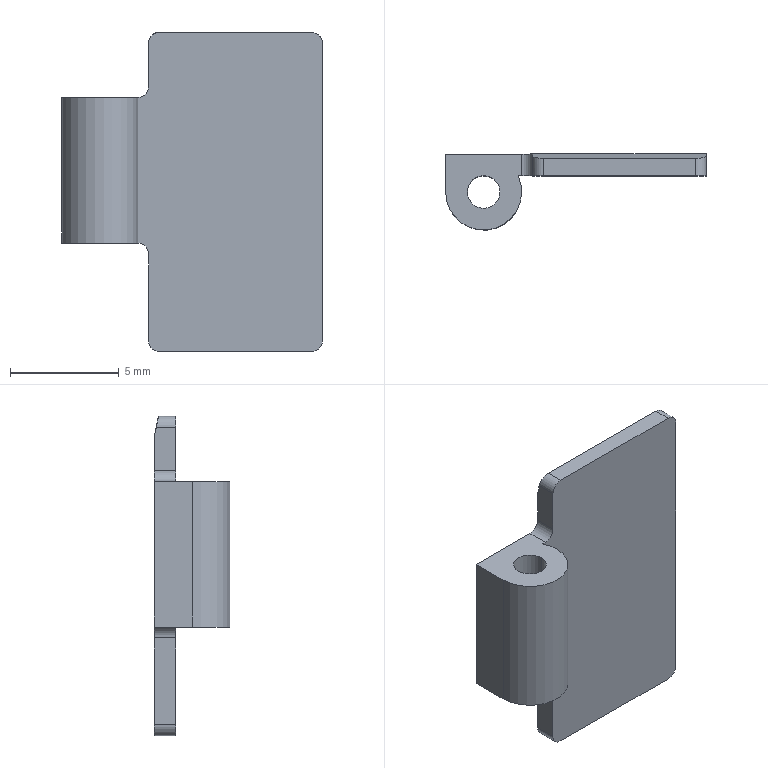Part | SolidWorks | features ICE 5, Chamfer 1, Extrusion 1, Fillet 1 | 1 solid | 20 faces | box 12 x 3.5 x 14.7 mm | volume 181.213 mm3 | plane 11 | cylinder 9 | commonest cylinder face diameters 1 x6 1.5 x2 3.5 x1
STEP:
#1=CARTESIAN_POINT('',(-0.75,0.,0.));
#2=VERTEX_POINT('',#1);
#3=CARTESIAN_POINT('',(0.75,0.,0.));
#4=VERTEX_POINT('',#3);
#5=CARTESIAN_POINT('',(0.,0.,0.));
#6=DIRECTION('',(0.,0.,1.));
#7=DIRECTION('',(1.,0.,0.));
#8=AXIS2_PLACEMENT_3D('',#5,#6,#7);
#9=CIRCLE('',#8,0.75);
#10=EDGE_CURVE('',#2,#4,#9,.T.);
#11=ORIENTED_EDGE('',*,*,#10,.F.);
#12=CARTESIAN_POINT('',(-0.75,0.,6.7));
#13=VERTEX_POINT('',#12);
#14=CARTESIAN_POINT('',(-0.75,0.,0.));
#15=DIRECTION('',(0.,0.,1.));
#16=VECTOR('',#15,1000.);
#17=LINE('',#14,#16);
#18=EDGE_CURVE('',#2,#13,#17,.T.);
#19=ORIENTED_EDGE('',*,*,#18,.T.);
#20=CARTESIAN_POINT('',(0.75,0.,6.7));
#21=VERTEX_POINT('',#20);
#22=CARTESIAN_POINT('',(0.,0.,6.7));
#23=DIRECTION('',(0.,0.,1.));
#24=DIRECTION('',(1.,0.,0.));
#25=AXIS2_PLACEMENT_3D('',#22,#23,#24);
#26=CIRCLE('',#25,0.75);
#27=EDGE_CURVE('',#13,#21,#26,.T.);
#28=ORIENTED_EDGE('',*,*,#27,.T.);
#29=CARTESIAN_POINT('',(0.75,0.,0.));
#30=DIRECTION('',(0.,0.,1.));
#31=VECTOR('',#30,1000.);
#32=LINE('',#29,#31);
#33=EDGE_CURVE('',#4,#21,#32,.T.);
#34=ORIENTED_EDGE('',*,*,#33,.F.);
#35=EDGE_LOOP('',(#11,#19,#28,#34));
#36=FACE_OUTER_BOUND('',#35,.T.);
#37=CARTESIAN_POINT('',(0.,0.,0.));
#38=DIRECTION('',(0.,0.,1.));
#39=DIRECTION('',(1.,0.,0.));
#40=AXIS2_PLACEMENT_3D('',#37,#38,#39);
#41=CYLINDRICAL_SURFACE('',#40,0.75);
#42=ADVANCED_FACE('',(#36),#41,.F.);
#43=CARTESIAN_POINT('',(0.,0.,0.));
#44=DIRECTION('',(0.,0.,1.));
#45=DIRECTION('',(1.,0.,0.));
#46=AXIS2_PLACEMENT_3D('',#43,#44,#45);
#47=CIRCLE('',#46,0.75);
#48=EDGE_CURVE('',#4,#2,#47,.T.);
#49=ORIENTED_EDGE('',*,*,#48,.T.);
#50=ORIENTED_EDGE('',*,*,#10,.T.);
#51=EDGE_LOOP('',(#49,#50));
#52=FACE_BOUND('',#51,.T.);
#53=CARTESIAN_POINT('',(1.75,1.75,0.));
#54=VERTEX_POINT('',#53);
#55=CARTESIAN_POINT('',(-1.75,1.75,0.));
#56=VERTEX_POINT('',#55);
#57=CARTESIAN_POINT('',(-1.75,1.75,0.));
#58=DIRECTION('',(-1.,0.,0.));
#59=VECTOR('',#58,1000.);
#60=LINE('',#57,#59);
#61=EDGE_CURVE('',#54,#56,#60,.T.);
#62=ORIENTED_EDGE('',*,*,#61,.F.);
#63=CARTESIAN_POINT('',(1.75,0.75,0.));
#64=VERTEX_POINT('',#63);
#65=CARTESIAN_POINT('',(1.75,0.75,0.));
#66=DIRECTION('',(0.,-1.,0.));
#67=VECTOR('',#66,1000.);
#68=LINE('',#65,#67);
#69=EDGE_CURVE('',#54,#64,#68,.T.);
#70=ORIENTED_EDGE('',*,*,#69,.T.);
#71=CARTESIAN_POINT('',(1.581,0.75,0.));
#72=VERTEX_POINT('',#71);
#73=CARTESIAN_POINT('',(-1.75,0.75,0.));
#74=DIRECTION('',(-1.,0.,0.));
#75=VECTOR('',#74,1000.);
#76=LINE('',#73,#75);
#77=EDGE_CURVE('',#64,#72,#76,.T.);
#78=ORIENTED_EDGE('',*,*,#77,.T.);
#79=CARTESIAN_POINT('',(-1.75,0.,0.));
#80=VERTEX_POINT('',#79);
#81=CARTESIAN_POINT('',(0.,0.,0.));
#82=DIRECTION('',(0.,0.,1.));
#83=DIRECTION('',(1.,0.,0.));
#84=AXIS2_PLACEMENT_3D('',#81,#82,#83);
#85=CIRCLE('',#84,1.75);
#86=EDGE_CURVE('',#80,#72,#85,.T.);
#87=ORIENTED_EDGE('',*,*,#86,.F.);
#88=CARTESIAN_POINT('',(-1.75,0.75,0.));
#89=DIRECTION('',(0.,1.,0.));
#90=VECTOR('',#89,1000.);
#91=LINE('',#88,#90);
#92=EDGE_CURVE('',#80,#56,#91,.T.);
#93=ORIENTED_EDGE('',*,*,#92,.T.);
#94=EDGE_LOOP('',(#62,#70,#78,#87,#93));
#95=FACE_OUTER_BOUND('',#94,.T.);
#96=CARTESIAN_POINT('',(0.,0.,0.));
#97=DIRECTION('',(0.,0.,1.));
#98=DIRECTION('',(1.,0.,0.));
#99=AXIS2_PLACEMENT_3D('',#96,#97,#98);
#100=PLANE('',#99);
#101=ADVANCED_FACE('',(#52,#95),#100,.F.);
#102=CARTESIAN_POINT('',(-1.75,0.,6.7));
#103=VERTEX_POINT('',#102);
#104=CARTESIAN_POINT('',(1.581,0.75,6.7));
#105=VERTEX_POINT('',#104);
#106=CARTESIAN_POINT('',(0.,0.,6.7));
#107=DIRECTION('',(0.,0.,1.));
#108=DIRECTION('',(1.,0.,0.));
#109=AXIS2_PLACEMENT_3D('',#106,#107,#108);
#110=CIRCLE('',#109,1.75);
#111=EDGE_CURVE('',#103,#105,#110,.T.);
#112=ORIENTED_EDGE('',*,*,#111,.F.);
#113=CARTESIAN_POINT('',(-1.75,0.,-0.7688));
#114=DIRECTION('',(0.,0.,1.));
#115=VECTOR('',#114,1000.);
#116=LINE('',#113,#115);
#117=EDGE_CURVE('',#80,#103,#116,.T.);
#118=ORIENTED_EDGE('',*,*,#117,.F.);
#119=ORIENTED_EDGE('',*,*,#86,.T.);
#120=CARTESIAN_POINT('',(1.581,0.75,6.7));
#121=DIRECTION('',(0.,0.,-1.));
#122=VECTOR('',#121,1000.);
#123=LINE('',#120,#122);
#124=EDGE_CURVE('',#105,#72,#123,.T.);
#125=ORIENTED_EDGE('',*,*,#124,.F.);
#126=EDGE_LOOP('',(#112,#118,#119,#125));
#127=FACE_OUTER_BOUND('',#126,.T.);
#128=CARTESIAN_POINT('',(0.,0.,6.7));
#129=DIRECTION('',(0.,0.,-1.));
#130=DIRECTION('',(-1.,0.,0.));
#131=AXIS2_PLACEMENT_3D('',#128,#129,#130);
#132=CYLINDRICAL_SURFACE('',#131,1.75);
#133=ADVANCED_FACE('',(#127),#132,.T.);
#134=CARTESIAN_POINT('',(1.75,0.75,6.7));
#135=VERTEX_POINT('',#134);
#136=CARTESIAN_POINT('',(-1.75,0.75,6.7));
#137=DIRECTION('',(1.,0.,0.));
#138=VECTOR('',#137,1000.);
#139=LINE('',#136,#138);
#140=EDGE_CURVE('',#105,#135,#139,.T.);
#141=ORIENTED_EDGE('',*,*,#140,.T.);
#142=CARTESIAN_POINT('',(1.75,1.75,6.7));
#143=VERTEX_POINT('',#142);
#144=CARTESIAN_POINT('',(1.75,0.,6.7));
#145=DIRECTION('',(0.,1.,0.));
#146=VECTOR('',#145,1000.);
#147=LINE('',#144,#146);
#148=EDGE_CURVE('',#135,#143,#147,.T.);
#149=ORIENTED_EDGE('',*,*,#148,.T.);
#150=CARTESIAN_POINT('',(-1.75,1.75,6.7));
#151=VERTEX_POINT('',#150);
#152=CARTESIAN_POINT('',(-1.75,1.75,6.7));
#153=DIRECTION('',(1.,0.,0.));
#154=VECTOR('',#153,1000.);
#155=LINE('',#152,#154);
#156=EDGE_CURVE('',#151,#143,#155,.T.);
#157=ORIENTED_EDGE('',*,*,#156,.F.);
#158=CARTESIAN_POINT('',(-1.75,0.75,6.7));
#159=DIRECTION('',(0.,1.,0.));
#160=VECTOR('',#159,1000.);
#161=LINE('',#158,#160);
#162=EDGE_CURVE('',#103,#151,#161,.T.);
#163=ORIENTED_EDGE('',*,*,#162,.F.);
#164=ORIENTED_EDGE('',*,*,#111,.T.);
#165=EDGE_LOOP('',(#141,#149,#157,#163,#164));
#166=FACE_OUTER_BOUND('',#165,.T.);
#167=CARTESIAN_POINT('',(0.,0.,6.7));
#168=DIRECTION('',(0.,0.,1.));
#169=DIRECTION('',(1.,0.,0.));
#170=AXIS2_PLACEMENT_3D('',#167,#168,#169);
#171=CIRCLE('',#170,0.75);
#172=EDGE_CURVE('',#21,#13,#171,.T.);
#173=ORIENTED_EDGE('',*,*,#172,.F.);
#174=ORIENTED_EDGE('',*,*,#27,.F.);
#175=EDGE_LOOP('',(#173,#174));
#176=FACE_BOUND('',#175,.T.);
#177=CARTESIAN_POINT('',(0.,0.,6.7));
#178=DIRECTION('',(0.,0.,1.));
#179=DIRECTION('',(1.,0.,0.));
#180=AXIS2_PLACEMENT_3D('',#177,#178,#179);
#181=PLANE('',#180);
#182=ADVANCED_FACE('',(#166,#176),#181,.T.);
#183=ORIENTED_EDGE('',*,*,#18,.F.);
#184=ORIENTED_EDGE('',*,*,#48,.F.);
#185=ORIENTED_EDGE('',*,*,#33,.T.);
#186=ORIENTED_EDGE('',*,*,#172,.T.);
#187=EDGE_LOOP('',(#183,#184,#185,#186));
#188=FACE_OUTER_BOUND('',#187,.T.);
#189=CARTESIAN_POINT('',(0.,0.,0.));
#190=DIRECTION('',(0.,0.,1.));
#191=DIRECTION('',(1.,0.,0.));
#192=AXIS2_PLACEMENT_3D('',#189,#190,#191);
#193=CYLINDRICAL_SURFACE('',#192,0.75);
#194=ADVANCED_FACE('',(#188),#193,.F.);
#195=CARTESIAN_POINT('',(2.75,1.75,-5.));
#196=VERTEX_POINT('',#195);
#197=CARTESIAN_POINT('',(9.75,1.75,-5.));
#198=VERTEX_POINT('',#197);
#199=CARTESIAN_POINT('',(2.25,1.75,-5.));
#200=DIRECTION('',(1.,0.,0.));
#201=VECTOR('',#200,1000.);
#202=LINE('',#199,#201);
#203=EDGE_CURVE('',#196,#198,#202,.T.);
#204=ORIENTED_EDGE('',*,*,#203,.F.);
#205=CARTESIAN_POINT('',(2.25,1.75,-4.5));
#206=VERTEX_POINT('',#205);
#207=CARTESIAN_POINT('',(2.75,1.75,-4.5));
#208=DIRECTION('',(0.,1.,0.));
#209=DIRECTION('',(0.,0.,1.));
#210=AXIS2_PLACEMENT_3D('',#207,#208,#209);
#211=CIRCLE('',#210,0.5);
#212=EDGE_CURVE('',#196,#206,#211,.T.);
#213=ORIENTED_EDGE('',*,*,#212,.T.);
#214=CARTESIAN_POINT('',(2.25,1.75,-0.5));
#215=VERTEX_POINT('',#214);
#216=CARTESIAN_POINT('',(2.25,1.75,-5.));
#217=DIRECTION('',(0.,0.,1.));
#218=VECTOR('',#217,1000.);
#219=LINE('',#216,#218);
#220=EDGE_CURVE('',#206,#215,#219,.T.);
#221=ORIENTED_EDGE('',*,*,#220,.T.);
#222=CARTESIAN_POINT('',(1.75,1.75,-0.5));
#223=DIRECTION('',(0.,-1.,0.));
#224=DIRECTION('',(0.,0.,1.));
#225=AXIS2_PLACEMENT_3D('',#222,#223,#224);
#226=CIRCLE('',#225,0.5);
#227=EDGE_CURVE('',#215,#54,#226,.T.);
#228=ORIENTED_EDGE('',*,*,#227,.T.);
#229=ORIENTED_EDGE('',*,*,#61,.T.);
#230=CARTESIAN_POINT('',(-1.75,1.75,0.));
#231=DIRECTION('',(0.,0.,1.));
#232=VECTOR('',#231,1000.);
#233=LINE('',#230,#232);
#234=EDGE_CURVE('',#56,#151,#233,.T.);
#235=ORIENTED_EDGE('',*,*,#234,.T.);
#236=ORIENTED_EDGE('',*,*,#156,.T.);
#237=CARTESIAN_POINT('',(2.25,1.75,7.2));
#238=VERTEX_POINT('',#237);
#239=CARTESIAN_POINT('',(1.75,1.75,7.2));
#240=DIRECTION('',(0.,-1.,0.));
#241=DIRECTION('',(0.,0.,1.));
#242=AXIS2_PLACEMENT_3D('',#239,#240,#241);
#243=CIRCLE('',#242,0.5);
#244=EDGE_CURVE('',#143,#238,#243,.T.);
#245=ORIENTED_EDGE('',*,*,#244,.T.);
#246=CARTESIAN_POINT('',(2.25,1.75,8.7));
#247=VERTEX_POINT('',#246);
#248=CARTESIAN_POINT('',(2.25,1.75,9.7));
#249=DIRECTION('',(0.,0.,-1.));
#250=VECTOR('',#249,1000.);
#251=LINE('',#248,#250);
#252=EDGE_CURVE('',#247,#238,#251,.T.);
#253=ORIENTED_EDGE('',*,*,#252,.F.);
#254=CARTESIAN_POINT('',(10.25,1.75,8.7));
#255=VERTEX_POINT('',#254);
#256=CARTESIAN_POINT('',(10.25,1.75,8.7));
#257=DIRECTION('',(1.,0.,0.));
#258=VECTOR('',#257,1000.);
#259=LINE('',#256,#258);
#260=EDGE_CURVE('',#247,#255,#259,.T.);
#261=ORIENTED_EDGE('',*,*,#260,.T.);
#262=CARTESIAN_POINT('',(10.25,1.75,-4.5));
#263=VERTEX_POINT('',#262);
#264=CARTESIAN_POINT('',(10.25,1.75,0.));
#265=DIRECTION('',(0.,0.,-1.));
#266=VECTOR('',#265,1000.);
#267=LINE('',#264,#266);
#268=EDGE_CURVE('',#255,#263,#267,.T.);
#269=ORIENTED_EDGE('',*,*,#268,.T.);
#270=CARTESIAN_POINT('',(9.75,1.75,-4.5));
#271=DIRECTION('',(0.,1.,0.));
#272=DIRECTION('',(0.,0.,1.));
#273=AXIS2_PLACEMENT_3D('',#270,#271,#272);
#274=CIRCLE('',#273,0.5);
#275=EDGE_CURVE('',#263,#198,#274,.T.);
#276=ORIENTED_EDGE('',*,*,#275,.T.);
#277=EDGE_LOOP('',(#204,#213,#221,#228,#229,#235,#236,#245,#253,#261,#269,#276));
#278=FACE_OUTER_BOUND('',#277,.T.);
#279=CARTESIAN_POINT('',(0.,1.75,0.));
#280=DIRECTION('',(0.,1.,0.));
#281=DIRECTION('',(0.,0.,1.));
#282=AXIS2_PLACEMENT_3D('',#279,#280,#281);
#283=PLANE('',#282);
#284=ADVANCED_FACE('',(#278),#283,.T.);
#285=CARTESIAN_POINT('',(10.25,0.75,9.2));
#286=VERTEX_POINT('',#285);
#287=CARTESIAN_POINT('',(10.25,0.75,-4.5));
#288=VERTEX_POINT('',#287);
#289=CARTESIAN_POINT('',(10.25,0.75,0.));
#290=DIRECTION('',(0.,0.,-1.));
#291=VECTOR('',#290,1000.);
#292=LINE('',#289,#291);
#293=EDGE_CURVE('',#286,#288,#292,.T.);
#294=ORIENTED_EDGE('',*,*,#293,.F.);
#295=CARTESIAN_POINT('',(9.75,0.75,9.7));
#296=VERTEX_POINT('',#295);
#297=CARTESIAN_POINT('',(9.75,0.75,9.2));
#298=DIRECTION('',(0.,-1.,0.));
#299=DIRECTION('',(0.,0.,1.));
#300=AXIS2_PLACEMENT_3D('',#297,#298,#299);
#301=CIRCLE('',#300,0.5);
#302=EDGE_CURVE('',#286,#296,#301,.T.);
#303=ORIENTED_EDGE('',*,*,#302,.T.);
#304=CARTESIAN_POINT('',(2.75,0.75,9.7));
#305=VERTEX_POINT('',#304);
#306=CARTESIAN_POINT('',(10.25,0.75,9.7));
#307=DIRECTION('',(1.,0.,0.));
#308=VECTOR('',#307,1000.);
#309=LINE('',#306,#308);
#310=EDGE_CURVE('',#305,#296,#309,.T.);
#311=ORIENTED_EDGE('',*,*,#310,.F.);
#312=CARTESIAN_POINT('',(2.25,0.75,9.2));
#313=VERTEX_POINT('',#312);
#314=CARTESIAN_POINT('',(2.75,0.75,9.2));
#315=DIRECTION('',(0.,-1.,0.));
#316=DIRECTION('',(0.,0.,1.));
#317=AXIS2_PLACEMENT_3D('',#314,#315,#316);
#318=CIRCLE('',#317,0.5);
#319=EDGE_CURVE('',#305,#313,#318,.T.);
#320=ORIENTED_EDGE('',*,*,#319,.T.);
#321=CARTESIAN_POINT('',(2.25,0.75,7.2));
#322=VERTEX_POINT('',#321);
#323=CARTESIAN_POINT('',(2.25,0.75,9.7));
#324=DIRECTION('',(0.,0.,-1.));
#325=VECTOR('',#324,1000.);
#326=LINE('',#323,#325);
#327=EDGE_CURVE('',#313,#322,#326,.T.);
#328=ORIENTED_EDGE('',*,*,#327,.T.);
#329=CARTESIAN_POINT('',(1.75,0.75,7.2));
#330=DIRECTION('',(0.,1.,0.));
#331=DIRECTION('',(0.,0.,1.));
#332=AXIS2_PLACEMENT_3D('',#329,#330,#331);
#333=CIRCLE('',#332,0.5);
#334=EDGE_CURVE('',#322,#135,#333,.T.);
#335=ORIENTED_EDGE('',*,*,#334,.T.);
#336=ORIENTED_EDGE('',*,*,#140,.F.);
#337=ORIENTED_EDGE('',*,*,#124,.T.);
#338=ORIENTED_EDGE('',*,*,#77,.F.);
#339=CARTESIAN_POINT('',(2.25,0.75,-0.5));
#340=VERTEX_POINT('',#339);
#341=CARTESIAN_POINT('',(1.75,0.75,-0.5));
#342=DIRECTION('',(0.,1.,0.));
#343=DIRECTION('',(0.,0.,1.));
#344=AXIS2_PLACEMENT_3D('',#341,#342,#343);
#345=CIRCLE('',#344,0.5);
#346=EDGE_CURVE('',#64,#340,#345,.T.);
#347=ORIENTED_EDGE('',*,*,#346,.T.);
#348=CARTESIAN_POINT('',(2.25,0.75,-4.5));
#349=VERTEX_POINT('',#348);
#350=CARTESIAN_POINT('',(2.25,0.75,-5.));
#351=DIRECTION('',(0.,0.,1.));
#352=VECTOR('',#351,1000.);
#353=LINE('',#350,#352);
#354=EDGE_CURVE('',#349,#340,#353,.T.);
#355=ORIENTED_EDGE('',*,*,#354,.F.);
#356=CARTESIAN_POINT('',(2.75,0.75,-5.));
#357=VERTEX_POINT('',#356);
#358=CARTESIAN_POINT('',(2.75,0.75,-4.5));
#359=DIRECTION('',(0.,-1.,0.));
#360=DIRECTION('',(0.,0.,1.));
#361=AXIS2_PLACEMENT_3D('',#358,#359,#360);
#362=CIRCLE('',#361,0.5);
#363=EDGE_CURVE('',#349,#357,#362,.T.);
#364=ORIENTED_EDGE('',*,*,#363,.T.);
#365=CARTESIAN_POINT('',(9.75,0.75,-5.));
#366=VERTEX_POINT('',#365);
#367=CARTESIAN_POINT('',(10.25,0.75,-5.));
#368=DIRECTION('',(-1.,0.,0.));
#369=VECTOR('',#368,1000.);
#370=LINE('',#367,#369);
#371=EDGE_CURVE('',#366,#357,#370,.T.);
#372=ORIENTED_EDGE('',*,*,#371,.F.);
#373=CARTESIAN_POINT('',(9.75,0.75,-4.5));
#374=DIRECTION('',(0.,-1.,0.));
#375=DIRECTION('',(0.,0.,1.));
#376=AXIS2_PLACEMENT_3D('',#373,#374,#375);
#377=CIRCLE('',#376,0.5);
#378=EDGE_CURVE('',#366,#288,#377,.T.);
#379=ORIENTED_EDGE('',*,*,#378,.T.);
#380=EDGE_LOOP('',(#294,#303,#311,#320,#328,#335,#336,#337,#338,#347,#355,#364,#372,#379));
#381=FACE_OUTER_BOUND('',#380,.T.);
#382=CARTESIAN_POINT('',(0.,0.75,0.));
#383=DIRECTION('',(0.,1.,0.));
#384=DIRECTION('',(0.,0.,1.));
#385=AXIS2_PLACEMENT_3D('',#382,#383,#384);
#386=PLANE('',#385);
#387=ADVANCED_FACE('',(#381),#386,.F.);
#388=ORIENTED_EDGE('',*,*,#234,.F.);
#389=ORIENTED_EDGE('',*,*,#92,.F.);
#390=ORIENTED_EDGE('',*,*,#117,.T.);
#391=ORIENTED_EDGE('',*,*,#162,.T.);
#392=EDGE_LOOP('',(#388,#389,#390,#391));
#393=FACE_OUTER_BOUND('',#392,.T.);
#394=CARTESIAN_POINT('',(-1.75,0.75,0.));
#395=DIRECTION('',(-1.,0.,0.));
#396=DIRECTION('',(0.,0.,1.));
#397=AXIS2_PLACEMENT_3D('',#394,#395,#396);
#398=PLANE('',#397);
#399=ADVANCED_FACE('',(#393),#398,.T.);
#400=CARTESIAN_POINT('',(10.25,1.65,9.2));
#401=VERTEX_POINT('',#400);
#402=CARTESIAN_POINT('',(10.25,3.385,0.5269));
#403=DIRECTION('',(0.,-0.1961,0.9806));
#404=VECTOR('',#403,1000.);
#405=LINE('',#402,#404);
#406=EDGE_CURVE('',#255,#401,#405,.T.);
#407=ORIENTED_EDGE('',*,*,#406,.T.);
#408=CARTESIAN_POINT('',(10.25,0.75,9.2));
#409=DIRECTION('',(0.,-1.,0.));
#410=VECTOR('',#409,1000.);
#411=LINE('',#408,#410);
#412=EDGE_CURVE('',#401,#286,#411,.T.);
#413=ORIENTED_EDGE('',*,*,#412,.T.);
#414=ORIENTED_EDGE('',*,*,#293,.T.);
#415=CARTESIAN_POINT('',(10.25,0.75,-4.5));
#416=DIRECTION('',(0.,1.,0.));
#417=VECTOR('',#416,1000.);
#418=LINE('',#415,#417);
#419=EDGE_CURVE('',#288,#263,#418,.T.);
#420=ORIENTED_EDGE('',*,*,#419,.T.);
#421=ORIENTED_EDGE('',*,*,#268,.F.);
#422=EDGE_LOOP('',(#407,#413,#414,#420,#421));
#423=FACE_OUTER_BOUND('',#422,.T.);
#424=CARTESIAN_POINT('',(10.25,0.75,0.));
#425=DIRECTION('',(1.,0.,0.));
#426=DIRECTION('',(0.,0.,-1.));
#427=AXIS2_PLACEMENT_3D('',#424,#425,#426);
#428=PLANE('',#427);
#429=ADVANCED_FACE('',(#423),#428,.T.);
#430=ORIENTED_EDGE('',*,*,#252,.T.);
#431=CARTESIAN_POINT('',(2.25,1.75,7.2));
#432=DIRECTION('',(0.,-1.,0.));
#433=VECTOR('',#432,1000.);
#434=LINE('',#431,#433);
#435=EDGE_CURVE('',#238,#322,#434,.T.);
#436=ORIENTED_EDGE('',*,*,#435,.T.);
#437=ORIENTED_EDGE('',*,*,#327,.F.);
#438=CARTESIAN_POINT('',(2.25,1.65,9.2));
#439=VERTEX_POINT('',#438);
#440=CARTESIAN_POINT('',(2.25,1.75,9.2));
#441=DIRECTION('',(0.,1.,0.));
#442=VECTOR('',#441,1000.);
#443=LINE('',#440,#442);
#444=EDGE_CURVE('',#313,#439,#443,.T.);
#445=ORIENTED_EDGE('',*,*,#444,.T.);
#446=CARTESIAN_POINT('',(2.25,1.55,9.7));
#447=DIRECTION('',(0.,0.1961,-0.9806));
#448=VECTOR('',#447,1000.);
#449=LINE('',#446,#448);
#450=EDGE_CURVE('',#439,#247,#449,.T.);
#451=ORIENTED_EDGE('',*,*,#450,.T.);
#452=EDGE_LOOP('',(#430,#436,#437,#445,#451));
#453=FACE_OUTER_BOUND('',#452,.T.);
#454=CARTESIAN_POINT('',(2.25,1.75,9.7));
#455=DIRECTION('',(1.,0.,0.));
#456=DIRECTION('',(0.,0.,-1.));
#457=AXIS2_PLACEMENT_3D('',#454,#455,#456);
#458=PLANE('',#457);
#459=ADVANCED_FACE('',(#453),#458,.F.);
#460=ORIENTED_EDGE('',*,*,#310,.T.);
#461=CARTESIAN_POINT('',(9.75,1.55,9.7));
#462=VERTEX_POINT('',#461);
#463=CARTESIAN_POINT('',(9.75,1.55,9.7));
#464=DIRECTION('',(0.,1.,0.));
#465=VECTOR('',#464,1000.);
#466=LINE('',#463,#465);
#467=EDGE_CURVE('',#296,#462,#466,.T.);
#468=ORIENTED_EDGE('',*,*,#467,.T.);
#469=CARTESIAN_POINT('',(2.75,1.55,9.7));
#470=VERTEX_POINT('',#469);
#471=CARTESIAN_POINT('',(2.25,1.55,9.7));
#472=DIRECTION('',(-1.,0.,0.));
#473=VECTOR('',#472,1000.);
#474=LINE('',#471,#473);
#475=EDGE_CURVE('',#462,#470,#474,.T.);
#476=ORIENTED_EDGE('',*,*,#475,.T.);
#477=CARTESIAN_POINT('',(2.75,0.,9.7));
#478=DIRECTION('',(0.,-1.,0.));
#479=VECTOR('',#478,1000.);
#480=LINE('',#477,#479);
#481=EDGE_CURVE('',#470,#305,#480,.T.);
#482=ORIENTED_EDGE('',*,*,#481,.T.);
#483=EDGE_LOOP('',(#460,#468,#476,#482));
#484=FACE_OUTER_BOUND('',#483,.T.);
#485=CARTESIAN_POINT('',(0.,0.,9.7));
#486=DIRECTION('',(0.,0.,-1.));
#487=DIRECTION('',(-1.,0.,0.));
#488=AXIS2_PLACEMENT_3D('',#485,#486,#487);
#489=PLANE('',#488);
#490=ADVANCED_FACE('',(#484),#489,.F.);
#491=ORIENTED_EDGE('',*,*,#354,.T.);
#492=CARTESIAN_POINT('',(2.25,1.75,-0.5));
#493=DIRECTION('',(0.,1.,0.));
#494=VECTOR('',#493,1000.);
#495=LINE('',#492,#494);
#496=EDGE_CURVE('',#340,#215,#495,.T.);
#497=ORIENTED_EDGE('',*,*,#496,.T.);
#498=ORIENTED_EDGE('',*,*,#220,.F.);
#499=CARTESIAN_POINT('',(2.25,0.75,-4.5));
#500=DIRECTION('',(0.,-1.,0.));
#501=VECTOR('',#500,1000.);
#502=LINE('',#499,#501);
#503=EDGE_CURVE('',#206,#349,#502,.T.);
#504=ORIENTED_EDGE('',*,*,#503,.T.);
#505=EDGE_LOOP('',(#491,#497,#498,#504));
#506=FACE_OUTER_BOUND('',#505,.T.);
#507=CARTESIAN_POINT('',(2.25,0.75,-5.));
#508=DIRECTION('',(1.,0.,0.));
#509=DIRECTION('',(0.,0.,-1.));
#510=AXIS2_PLACEMENT_3D('',#507,#508,#509);
#511=PLANE('',#510);
#512=ADVANCED_FACE('',(#506),#511,.F.);
#513=ORIENTED_EDGE('',*,*,#371,.T.);
#514=CARTESIAN_POINT('',(2.75,1.75,-5.));
#515=DIRECTION('',(0.,1.,0.));
#516=VECTOR('',#515,1000.);
#517=LINE('',#514,#516);
#518=EDGE_CURVE('',#357,#196,#517,.T.);
#519=ORIENTED_EDGE('',*,*,#518,.T.);
#520=ORIENTED_EDGE('',*,*,#203,.T.);
#521=CARTESIAN_POINT('',(9.75,0.,-5.));
#522=DIRECTION('',(0.,-1.,0.));
#523=VECTOR('',#522,1000.);
#524=LINE('',#521,#523);
#525=EDGE_CURVE('',#198,#366,#524,.T.);
#526=ORIENTED_EDGE('',*,*,#525,.T.);
#527=EDGE_LOOP('',(#513,#519,#520,#526));
#528=FACE_OUTER_BOUND('',#527,.T.);
#529=CARTESIAN_POINT('',(0.,0.,-5.));
#530=DIRECTION('',(0.,0.,-1.));
#531=DIRECTION('',(-1.,0.,0.));
#532=AXIS2_PLACEMENT_3D('',#529,#530,#531);
#533=PLANE('',#532);
#534=ADVANCED_FACE('',(#528),#533,.T.);
#535=ORIENTED_EDGE('',*,*,#475,.F.);
#536=CARTESIAN_POINT('',(9.75,1.55,9.7));
#537=CARTESIAN_POINT('',(10.043,1.55,9.7));
#538=CARTESIAN_POINT('',(10.25,1.591,9.493));
#539=CARTESIAN_POINT('',(10.25,1.65,9.2));
#540=(BOUNDED_CURVE()B_SPLINE_CURVE(3,(#536,#537,#538,#539),.UNSPECIFIED.,.F.,.F.)B_SPLINE_CURVE_WITH_KNOTS((4,4),(0.,1.571),.UNSPECIFIED.)CURVE()GEOMETRIC_REPRESENTATION_ITEM()RATIONAL_B_SPLINE_CURVE((1.,0.8047,0.8047,1.))REPRESENTATION_ITEM(''));
#541=EDGE_CURVE('',#462,#401,#540,.T.);
#542=ORIENTED_EDGE('',*,*,#541,.T.);
#543=ORIENTED_EDGE('',*,*,#406,.F.);
#544=ORIENTED_EDGE('',*,*,#260,.F.);
#545=ORIENTED_EDGE('',*,*,#450,.F.);
#546=CARTESIAN_POINT('',(2.25,1.65,9.2));
#547=CARTESIAN_POINT('',(2.25,1.591,9.493));
#548=CARTESIAN_POINT('',(2.457,1.55,9.7));
#549=CARTESIAN_POINT('',(2.75,1.55,9.7));
#550=(BOUNDED_CURVE()B_SPLINE_CURVE(3,(#546,#547,#548,#549),.UNSPECIFIED.,.F.,.F.)B_SPLINE_CURVE_WITH_KNOTS((4,4),(4.712,6.283),.UNSPECIFIED.)CURVE()GEOMETRIC_REPRESENTATION_ITEM()RATIONAL_B_SPLINE_CURVE((1.,0.8047,0.8047,1.))REPRESENTATION_ITEM(''));
#551=EDGE_CURVE('',#439,#470,#550,.T.);
#552=ORIENTED_EDGE('',*,*,#551,.T.);
#553=EDGE_LOOP('',(#535,#542,#543,#544,#545,#552));
#554=FACE_OUTER_BOUND('',#553,.T.);
#555=CARTESIAN_POINT('',(0.,1.55,9.7));
#556=DIRECTION('',(0.,0.9806,0.1961));
#557=DIRECTION('',(1.,0.,0.));
#558=AXIS2_PLACEMENT_3D('',#555,#556,#557);
#559=PLANE('',#558);
#560=ADVANCED_FACE('',(#554),#559,.T.);
#561=ORIENTED_EDGE('',*,*,#244,.F.);
#562=ORIENTED_EDGE('',*,*,#148,.F.);
#563=ORIENTED_EDGE('',*,*,#334,.F.);
#564=ORIENTED_EDGE('',*,*,#435,.F.);
#565=EDGE_LOOP('',(#561,#562,#563,#564));
#566=FACE_OUTER_BOUND('',#565,.T.);
#567=CARTESIAN_POINT('',(1.75,1.75,7.2));
#568=DIRECTION('',(0.,-1.,0.));
#569=DIRECTION('',(0.,0.,-1.));
#570=AXIS2_PLACEMENT_3D('',#567,#568,#569);
#571=CYLINDRICAL_SURFACE('',#570,0.5);
#572=ADVANCED_FACE('',(#566),#571,.F.);
#573=ORIENTED_EDGE('',*,*,#346,.F.);
#574=ORIENTED_EDGE('',*,*,#69,.F.);
#575=ORIENTED_EDGE('',*,*,#227,.F.);
#576=ORIENTED_EDGE('',*,*,#496,.F.);
#577=EDGE_LOOP('',(#573,#574,#575,#576));
#578=FACE_OUTER_BOUND('',#577,.T.);
#579=CARTESIAN_POINT('',(1.75,0.75,-0.5));
#580=DIRECTION('',(0.,-1.,0.));
#581=DIRECTION('',(0.,0.,-1.));
#582=AXIS2_PLACEMENT_3D('',#579,#580,#581);
#583=CYLINDRICAL_SURFACE('',#582,0.5);
#584=ADVANCED_FACE('',(#578),#583,.F.);
#585=ORIENTED_EDGE('',*,*,#302,.F.);
#586=ORIENTED_EDGE('',*,*,#412,.F.);
#587=ORIENTED_EDGE('',*,*,#541,.F.);
#588=ORIENTED_EDGE('',*,*,#467,.F.);
#589=EDGE_LOOP('',(#585,#586,#587,#588));
#590=FACE_OUTER_BOUND('',#589,.T.);
#591=CARTESIAN_POINT('',(9.75,0.,9.2));
#592=DIRECTION('',(0.,-1.,0.));
#593=DIRECTION('',(0.,0.,-1.));
#594=AXIS2_PLACEMENT_3D('',#591,#592,#593);
#595=CYLINDRICAL_SURFACE('',#594,0.5);
#596=ADVANCED_FACE('',(#590),#595,.T.);
#597=ORIENTED_EDGE('',*,*,#551,.F.);
#598=ORIENTED_EDGE('',*,*,#444,.F.);
#599=ORIENTED_EDGE('',*,*,#319,.F.);
#600=ORIENTED_EDGE('',*,*,#481,.F.);
#601=EDGE_LOOP('',(#597,#598,#599,#600));
#602=FACE_OUTER_BOUND('',#601,.T.);
#603=CARTESIAN_POINT('',(2.75,0.,9.2));
#604=DIRECTION('',(0.,-1.,0.));
#605=DIRECTION('',(0.,0.,-1.));
#606=AXIS2_PLACEMENT_3D('',#603,#604,#605);
#607=CYLINDRICAL_SURFACE('',#606,0.5);
#608=ADVANCED_FACE('',(#602),#607,.T.);
#609=ORIENTED_EDGE('',*,*,#363,.F.);
#610=ORIENTED_EDGE('',*,*,#503,.F.);
#611=ORIENTED_EDGE('',*,*,#212,.F.);
#612=ORIENTED_EDGE('',*,*,#518,.F.);
#613=EDGE_LOOP('',(#609,#610,#611,#612));
#614=FACE_OUTER_BOUND('',#613,.T.);
#615=CARTESIAN_POINT('',(2.75,0.,-4.5));
#616=DIRECTION('',(0.,-1.,0.));
#617=DIRECTION('',(0.,0.,-1.));
#618=AXIS2_PLACEMENT_3D('',#615,#616,#617);
#619=CYLINDRICAL_SURFACE('',#618,0.5);
#620=ADVANCED_FACE('',(#614),#619,.T.);
#621=ORIENTED_EDGE('',*,*,#275,.F.);
#622=ORIENTED_EDGE('',*,*,#419,.F.);
#623=ORIENTED_EDGE('',*,*,#378,.F.);
#624=ORIENTED_EDGE('',*,*,#525,.F.);
#625=EDGE_LOOP('',(#621,#622,#623,#624));
#626=FACE_OUTER_BOUND('',#625,.T.);
#627=CARTESIAN_POINT('',(9.75,0.,-4.5));
#628=DIRECTION('',(0.,-1.,0.));
#629=DIRECTION('',(0.,0.,-1.));
#630=AXIS2_PLACEMENT_3D('',#627,#628,#629);
#631=CYLINDRICAL_SURFACE('',#630,0.5);
#632=ADVANCED_FACE('',(#626),#631,.T.);
#633=CLOSED_SHELL('',(#42,#101,#133,#182,#194,#284,#387,#399,#429,#459,#490,#512,#534,#560,#572,#584,#596,#608,#620,#632));
#634=MANIFOLD_SOLID_BREP('',#633);
#635=CARTESIAN_POINT('',(0.,0.,0.));
#636=DIRECTION('',(0.,0.,1.));
#637=DIRECTION('',(1.,0.,0.));
#638=AXIS2_PLACEMENT_3D('',#635,#636,#637);
#639=(LENGTH_UNIT()NAMED_UNIT(*)SI_UNIT(.MILLI.,.METRE.));
#640=UNCERTAINTY_MEASURE_WITH_UNIT(LENGTH_MEASURE(0.00001),#639,'','');
#641=(NAMED_UNIT(*)PLANE_ANGLE_UNIT()SI_UNIT($,.RADIAN.));
#642=(NAMED_UNIT(*)SI_UNIT($,.STERADIAN.)SOLID_ANGLE_UNIT());
#643=(GEOMETRIC_REPRESENTATION_CONTEXT(3)GLOBAL_UNCERTAINTY_ASSIGNED_CONTEXT((#640))GLOBAL_UNIT_ASSIGNED_CONTEXT((#639,#641,#642))REPRESENTATION_CONTEXT('',''));
#644=ADVANCED_BREP_SHAPE_REPRESENTATION('',(#634,#638),#643);